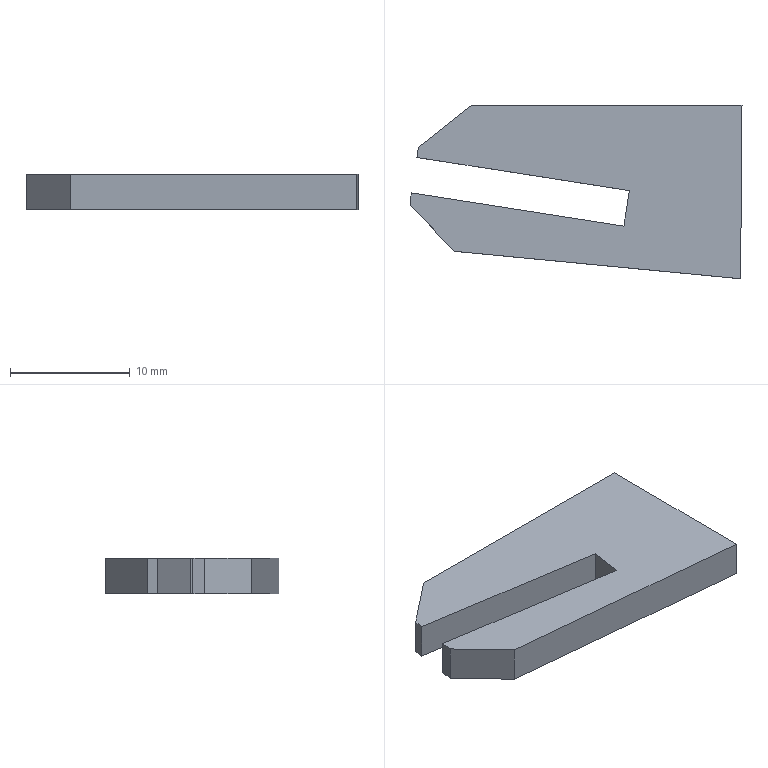Part | SolidWorks | features BaseBody 1 | 1 solid | 12 faces | box 27.749 x 14.503 x 3 mm | volume 877.652 mm3 | plane 12
STEP:
#1=CARTESIAN_POINT('',(-15.417,90.586,-1.5));
#2=VERTEX_POINT('',#1);
#3=CARTESIAN_POINT('',(-19.116,94.481,-1.5));
#4=VERTEX_POINT('',#3);
#5=CARTESIAN_POINT('',(37.126,35.256,-1.5));
#6=DIRECTION('',(-0.6886,0.7251,0.));
#7=VECTOR('',#6,1000.);
#8=LINE('',#5,#7);
#9=EDGE_CURVE('',#2,#4,#8,.T.);
#10=ORIENTED_EDGE('',*,*,#9,.T.);
#11=CARTESIAN_POINT('',(-19.007,95.47,-1.5));
#12=VERTEX_POINT('',#11);
#13=CARTESIAN_POINT('',(-29.164,3.211,-1.5));
#14=DIRECTION('',(0.1094,0.994,0.));
#15=VECTOR('',#14,1000.);
#16=LINE('',#13,#15);
#17=EDGE_CURVE('',#4,#12,#16,.T.);
#18=ORIENTED_EDGE('',*,*,#17,.T.);
#19=CARTESIAN_POINT('',(-1.242,92.691,-1.5));
#20=VERTEX_POINT('',#19);
#21=CARTESIAN_POINT('',(14.126,90.286,-1.5));
#22=DIRECTION('',(0.988,-0.1546,0.));
#23=VECTOR('',#22,1000.);
#24=LINE('',#21,#23);
#25=EDGE_CURVE('',#12,#20,#24,.T.);
#26=ORIENTED_EDGE('',*,*,#25,.T.);
#27=CARTESIAN_POINT('',(-0.7787,95.655,-1.5));
#28=VERTEX_POINT('',#27);
#29=CARTESIAN_POINT('',(-15.369,2.405,-1.5));
#30=DIRECTION('',(-0.1546,-0.988,0.));
#31=VECTOR('',#30,1000.);
#32=LINE('',#29,#31);
#33=EDGE_CURVE('',#28,#20,#32,.T.);
#34=ORIENTED_EDGE('',*,*,#33,.F.);
#35=CARTESIAN_POINT('',(-18.541,98.434,-1.5));
#36=VERTEX_POINT('',#35);
#37=CARTESIAN_POINT('',(14.59,93.25,-1.5));
#38=DIRECTION('',(0.988,-0.1546,0.));
#39=VECTOR('',#38,1000.);
#40=LINE('',#37,#39);
#41=EDGE_CURVE('',#36,#28,#40,.T.);
#42=ORIENTED_EDGE('',*,*,#41,.F.);
#43=CARTESIAN_POINT('',(-18.41,99.272,-1.5));
#44=VERTEX_POINT('',#43);
#45=CARTESIAN_POINT('',(-33.113,5.174,-1.5));
#46=DIRECTION('',(-0.1544,-0.988,0.));
#47=VECTOR('',#46,1000.);
#48=LINE('',#45,#47);
#49=EDGE_CURVE('',#44,#36,#48,.T.);
#50=ORIENTED_EDGE('',*,*,#49,.F.);
#51=CARTESIAN_POINT('',(-13.951,102.794,-1.5));
#52=VERTEX_POINT('',#51);
#53=CARTESIAN_POINT('',(-55.356,70.096,-1.5));
#54=DIRECTION('',(-0.7848,-0.6198,0.));
#55=VECTOR('',#54,1000.);
#56=LINE('',#53,#55);
#57=EDGE_CURVE('',#52,#44,#56,.T.);
#58=ORIENTED_EDGE('',*,*,#57,.F.);
#59=CARTESIAN_POINT('',(8.633,102.795,-1.5));
#60=VERTEX_POINT('',#59);
#61=CARTESIAN_POINT('',(-0.006828,102.795,-1.5));
#62=DIRECTION('',(1.,0.00006642,0.));
#63=VECTOR('',#62,1000.);
#64=LINE('',#61,#63);
#65=EDGE_CURVE('',#52,#60,#64,.T.);
#66=ORIENTED_EDGE('',*,*,#65,.T.);
#67=CARTESIAN_POINT('',(8.515,88.292,-1.5));
#68=VERTEX_POINT('',#67);
#69=CARTESIAN_POINT('',(7.797,-0.06338,-1.5));
#70=DIRECTION('',(0.008129,1.,0.));
#71=VECTOR('',#70,1000.);
#72=LINE('',#69,#71);
#73=EDGE_CURVE('',#68,#60,#72,.T.);
#74=ORIENTED_EDGE('',*,*,#73,.F.);
#75=CARTESIAN_POINT('',(8.464,88.297,-1.5));
#76=DIRECTION('',(0.9954,-0.09542,0.));
#77=VECTOR('',#76,1000.);
#78=LINE('',#75,#77);
#79=EDGE_CURVE('',#2,#68,#78,.T.);
#80=ORIENTED_EDGE('',*,*,#79,.F.);
#81=EDGE_LOOP('',(#10,#18,#26,#34,#42,#50,#58,#66,#74,#80));
#82=FACE_OUTER_BOUND('',#81,.T.);
#83=CARTESIAN_POINT('',(0.,0.,-1.5));
#84=DIRECTION('',(0.,0.,1.));
#85=DIRECTION('',(1.,0.,0.));
#86=AXIS2_PLACEMENT_3D('',#83,#84,#85);
#87=PLANE('',#86);
#88=ADVANCED_FACE('',(#82),#87,.F.);
#89=CARTESIAN_POINT('',(-15.417,90.586,1.5));
#90=VERTEX_POINT('',#89);
#91=CARTESIAN_POINT('',(-19.116,94.481,1.5));
#92=VERTEX_POINT('',#91);
#93=CARTESIAN_POINT('',(37.126,35.256,1.5));
#94=DIRECTION('',(-0.6886,0.7251,0.));
#95=VECTOR('',#94,1000.);
#96=LINE('',#93,#95);
#97=EDGE_CURVE('',#90,#92,#96,.T.);
#98=ORIENTED_EDGE('',*,*,#97,.F.);
#99=CARTESIAN_POINT('',(8.515,88.292,1.5));
#100=VERTEX_POINT('',#99);
#101=CARTESIAN_POINT('',(8.464,88.297,1.5));
#102=DIRECTION('',(0.9954,-0.09542,0.));
#103=VECTOR('',#102,1000.);
#104=LINE('',#101,#103);
#105=EDGE_CURVE('',#90,#100,#104,.T.);
#106=ORIENTED_EDGE('',*,*,#105,.T.);
#107=CARTESIAN_POINT('',(8.633,102.795,1.5));
#108=VERTEX_POINT('',#107);
#109=CARTESIAN_POINT('',(7.797,-0.06338,1.5));
#110=DIRECTION('',(0.008129,1.,0.));
#111=VECTOR('',#110,1000.);
#112=LINE('',#109,#111);
#113=EDGE_CURVE('',#100,#108,#112,.T.);
#114=ORIENTED_EDGE('',*,*,#113,.T.);
#115=CARTESIAN_POINT('',(-13.951,102.794,1.5));
#116=VERTEX_POINT('',#115);
#117=CARTESIAN_POINT('',(-0.006828,102.795,1.5));
#118=DIRECTION('',(1.,0.00006642,0.));
#119=VECTOR('',#118,1000.);
#120=LINE('',#117,#119);
#121=EDGE_CURVE('',#116,#108,#120,.T.);
#122=ORIENTED_EDGE('',*,*,#121,.F.);
#123=CARTESIAN_POINT('',(-18.41,99.272,1.5));
#124=VERTEX_POINT('',#123);
#125=CARTESIAN_POINT('',(-55.356,70.096,1.5));
#126=DIRECTION('',(-0.7848,-0.6198,0.));
#127=VECTOR('',#126,1000.);
#128=LINE('',#125,#127);
#129=EDGE_CURVE('',#116,#124,#128,.T.);
#130=ORIENTED_EDGE('',*,*,#129,.T.);
#131=CARTESIAN_POINT('',(-18.541,98.434,1.5));
#132=VERTEX_POINT('',#131);
#133=CARTESIAN_POINT('',(-33.113,5.174,1.5));
#134=DIRECTION('',(-0.1544,-0.988,0.));
#135=VECTOR('',#134,1000.);
#136=LINE('',#133,#135);
#137=EDGE_CURVE('',#124,#132,#136,.T.);
#138=ORIENTED_EDGE('',*,*,#137,.T.);
#139=CARTESIAN_POINT('',(-0.7787,95.655,1.5));
#140=VERTEX_POINT('',#139);
#141=CARTESIAN_POINT('',(14.59,93.25,1.5));
#142=DIRECTION('',(0.988,-0.1546,0.));
#143=VECTOR('',#142,1000.);
#144=LINE('',#141,#143);
#145=EDGE_CURVE('',#132,#140,#144,.T.);
#146=ORIENTED_EDGE('',*,*,#145,.T.);
#147=CARTESIAN_POINT('',(-1.242,92.691,1.5));
#148=VERTEX_POINT('',#147);
#149=CARTESIAN_POINT('',(-15.369,2.405,1.5));
#150=DIRECTION('',(-0.1546,-0.988,0.));
#151=VECTOR('',#150,1000.);
#152=LINE('',#149,#151);
#153=EDGE_CURVE('',#140,#148,#152,.T.);
#154=ORIENTED_EDGE('',*,*,#153,.T.);
#155=CARTESIAN_POINT('',(-19.007,95.47,1.5));
#156=VERTEX_POINT('',#155);
#157=CARTESIAN_POINT('',(14.126,90.286,1.5));
#158=DIRECTION('',(0.988,-0.1546,0.));
#159=VECTOR('',#158,1000.);
#160=LINE('',#157,#159);
#161=EDGE_CURVE('',#156,#148,#160,.T.);
#162=ORIENTED_EDGE('',*,*,#161,.F.);
#163=CARTESIAN_POINT('',(-29.164,3.211,1.5));
#164=DIRECTION('',(0.1094,0.994,0.));
#165=VECTOR('',#164,1000.);
#166=LINE('',#163,#165);
#167=EDGE_CURVE('',#92,#156,#166,.T.);
#168=ORIENTED_EDGE('',*,*,#167,.F.);
#169=EDGE_LOOP('',(#98,#106,#114,#122,#130,#138,#146,#154,#162,#168));
#170=FACE_OUTER_BOUND('',#169,.T.);
#171=CARTESIAN_POINT('',(0.,0.,1.5));
#172=DIRECTION('',(0.,0.,1.));
#173=DIRECTION('',(1.,0.,0.));
#174=AXIS2_PLACEMENT_3D('',#171,#172,#173);
#175=PLANE('',#174);
#176=ADVANCED_FACE('',(#170),#175,.T.);
#177=ORIENTED_EDGE('',*,*,#17,.F.);
#178=CARTESIAN_POINT('',(-19.116,94.481,1.5));
#179=DIRECTION('',(0.,0.,-1.));
#180=VECTOR('',#179,1000.);
#181=LINE('',#178,#180);
#182=EDGE_CURVE('',#92,#4,#181,.T.);
#183=ORIENTED_EDGE('',*,*,#182,.F.);
#184=ORIENTED_EDGE('',*,*,#167,.T.);
#185=CARTESIAN_POINT('',(-19.007,95.47,1.5));
#186=DIRECTION('',(0.,0.,-1.));
#187=VECTOR('',#186,1000.);
#188=LINE('',#185,#187);
#189=EDGE_CURVE('',#156,#12,#188,.T.);
#190=ORIENTED_EDGE('',*,*,#189,.T.);
#191=EDGE_LOOP('',(#177,#183,#184,#190));
#192=FACE_OUTER_BOUND('',#191,.T.);
#193=CARTESIAN_POINT('',(-29.164,3.211,1.5));
#194=DIRECTION('',(-0.994,0.1094,0.));
#195=DIRECTION('',(0.,0.,1.));
#196=AXIS2_PLACEMENT_3D('',#193,#194,#195);
#197=PLANE('',#196);
#198=ADVANCED_FACE('',(#192),#197,.T.);
#199=ORIENTED_EDGE('',*,*,#25,.F.);
#200=ORIENTED_EDGE('',*,*,#189,.F.);
#201=ORIENTED_EDGE('',*,*,#161,.T.);
#202=CARTESIAN_POINT('',(-1.242,92.691,1.5));
#203=DIRECTION('',(0.,0.,-1.));
#204=VECTOR('',#203,1000.);
#205=LINE('',#202,#204);
#206=EDGE_CURVE('',#148,#20,#205,.T.);
#207=ORIENTED_EDGE('',*,*,#206,.T.);
#208=EDGE_LOOP('',(#199,#200,#201,#207));
#209=FACE_OUTER_BOUND('',#208,.T.);
#210=CARTESIAN_POINT('',(14.126,90.286,1.5));
#211=DIRECTION('',(0.1546,0.988,0.));
#212=DIRECTION('',(0.,0.,-1.));
#213=AXIS2_PLACEMENT_3D('',#210,#211,#212);
#214=PLANE('',#213);
#215=ADVANCED_FACE('',(#209),#214,.T.);
#216=ORIENTED_EDGE('',*,*,#33,.T.);
#217=ORIENTED_EDGE('',*,*,#206,.F.);
#218=ORIENTED_EDGE('',*,*,#153,.F.);
#219=CARTESIAN_POINT('',(-0.7787,95.655,1.5));
#220=DIRECTION('',(0.,0.,-1.));
#221=VECTOR('',#220,1000.);
#222=LINE('',#219,#221);
#223=EDGE_CURVE('',#140,#28,#222,.T.);
#224=ORIENTED_EDGE('',*,*,#223,.T.);
#225=EDGE_LOOP('',(#216,#217,#218,#224));
#226=FACE_OUTER_BOUND('',#225,.T.);
#227=CARTESIAN_POINT('',(-15.369,2.405,1.5));
#228=DIRECTION('',(0.988,-0.1546,0.));
#229=DIRECTION('',(0.,0.,-1.));
#230=AXIS2_PLACEMENT_3D('',#227,#228,#229);
#231=PLANE('',#230);
#232=ADVANCED_FACE('',(#226),#231,.F.);
#233=ORIENTED_EDGE('',*,*,#41,.T.);
#234=ORIENTED_EDGE('',*,*,#223,.F.);
#235=ORIENTED_EDGE('',*,*,#145,.F.);
#236=CARTESIAN_POINT('',(-18.541,98.434,1.5));
#237=DIRECTION('',(0.,0.,-1.));
#238=VECTOR('',#237,1000.);
#239=LINE('',#236,#238);
#240=EDGE_CURVE('',#132,#36,#239,.T.);
#241=ORIENTED_EDGE('',*,*,#240,.T.);
#242=EDGE_LOOP('',(#233,#234,#235,#241));
#243=FACE_OUTER_BOUND('',#242,.T.);
#244=CARTESIAN_POINT('',(14.59,93.25,1.5));
#245=DIRECTION('',(0.1546,0.988,0.));
#246=DIRECTION('',(0.,0.,-1.));
#247=AXIS2_PLACEMENT_3D('',#244,#245,#246);
#248=PLANE('',#247);
#249=ADVANCED_FACE('',(#243),#248,.F.);
#250=ORIENTED_EDGE('',*,*,#49,.T.);
#251=ORIENTED_EDGE('',*,*,#240,.F.);
#252=ORIENTED_EDGE('',*,*,#137,.F.);
#253=CARTESIAN_POINT('',(-18.41,99.272,1.5));
#254=DIRECTION('',(0.,0.,-1.));
#255=VECTOR('',#254,1000.);
#256=LINE('',#253,#255);
#257=EDGE_CURVE('',#124,#44,#256,.T.);
#258=ORIENTED_EDGE('',*,*,#257,.T.);
#259=EDGE_LOOP('',(#250,#251,#252,#258));
#260=FACE_OUTER_BOUND('',#259,.T.);
#261=CARTESIAN_POINT('',(-33.113,5.174,1.5));
#262=DIRECTION('',(0.988,-0.1544,0.));
#263=DIRECTION('',(0.,0.,-1.));
#264=AXIS2_PLACEMENT_3D('',#261,#262,#263);
#265=PLANE('',#264);
#266=ADVANCED_FACE('',(#260),#265,.F.);
#267=ORIENTED_EDGE('',*,*,#57,.T.);
#268=ORIENTED_EDGE('',*,*,#257,.F.);
#269=ORIENTED_EDGE('',*,*,#129,.F.);
#270=CARTESIAN_POINT('',(-13.951,102.794,1.5));
#271=DIRECTION('',(0.,0.,-1.));
#272=VECTOR('',#271,1000.);
#273=LINE('',#270,#272);
#274=EDGE_CURVE('',#116,#52,#273,.T.);
#275=ORIENTED_EDGE('',*,*,#274,.T.);
#276=EDGE_LOOP('',(#267,#268,#269,#275));
#277=FACE_OUTER_BOUND('',#276,.T.);
#278=CARTESIAN_POINT('',(-55.356,70.096,1.5));
#279=DIRECTION('',(0.6198,-0.7848,0.));
#280=DIRECTION('',(0.,0.,-1.));
#281=AXIS2_PLACEMENT_3D('',#278,#279,#280);
#282=PLANE('',#281);
#283=ADVANCED_FACE('',(#277),#282,.F.);
#284=ORIENTED_EDGE('',*,*,#65,.F.);
#285=ORIENTED_EDGE('',*,*,#274,.F.);
#286=ORIENTED_EDGE('',*,*,#121,.T.);
#287=CARTESIAN_POINT('',(8.633,102.795,1.5));
#288=DIRECTION('',(0.,0.,-1.));
#289=VECTOR('',#288,1000.);
#290=LINE('',#287,#289);
#291=EDGE_CURVE('',#108,#60,#290,.T.);
#292=ORIENTED_EDGE('',*,*,#291,.T.);
#293=EDGE_LOOP('',(#284,#285,#286,#292));
#294=FACE_OUTER_BOUND('',#293,.T.);
#295=CARTESIAN_POINT('',(-0.006828,102.795,1.5));
#296=DIRECTION('',(-0.00006642,1.,0.));
#297=DIRECTION('',(0.,0.,1.));
#298=AXIS2_PLACEMENT_3D('',#295,#296,#297);
#299=PLANE('',#298);
#300=ADVANCED_FACE('',(#294),#299,.T.);
#301=ORIENTED_EDGE('',*,*,#73,.T.);
#302=ORIENTED_EDGE('',*,*,#291,.F.);
#303=ORIENTED_EDGE('',*,*,#113,.F.);
#304=CARTESIAN_POINT('',(8.515,88.292,1.5));
#305=DIRECTION('',(0.,0.,-1.));
#306=VECTOR('',#305,1000.);
#307=LINE('',#304,#306);
#308=EDGE_CURVE('',#100,#68,#307,.T.);
#309=ORIENTED_EDGE('',*,*,#308,.T.);
#310=EDGE_LOOP('',(#301,#302,#303,#309));
#311=FACE_OUTER_BOUND('',#310,.T.);
#312=CARTESIAN_POINT('',(7.797,-0.06338,1.5));
#313=DIRECTION('',(-1.,0.008129,0.));
#314=DIRECTION('',(0.,0.,1.));
#315=AXIS2_PLACEMENT_3D('',#312,#313,#314);
#316=PLANE('',#315);
#317=ADVANCED_FACE('',(#311),#316,.F.);
#318=ORIENTED_EDGE('',*,*,#79,.T.);
#319=ORIENTED_EDGE('',*,*,#308,.F.);
#320=ORIENTED_EDGE('',*,*,#105,.F.);
#321=CARTESIAN_POINT('',(-15.417,90.586,1.5));
#322=DIRECTION('',(0.,0.,-1.));
#323=VECTOR('',#322,1000.);
#324=LINE('',#321,#323);
#325=EDGE_CURVE('',#90,#2,#324,.T.);
#326=ORIENTED_EDGE('',*,*,#325,.T.);
#327=EDGE_LOOP('',(#318,#319,#320,#326));
#328=FACE_OUTER_BOUND('',#327,.T.);
#329=CARTESIAN_POINT('',(8.464,88.297,1.5));
#330=DIRECTION('',(0.09542,0.9954,0.));
#331=DIRECTION('',(0.,0.,-1.));
#332=AXIS2_PLACEMENT_3D('',#329,#330,#331);
#333=PLANE('',#332);
#334=ADVANCED_FACE('',(#328),#333,.F.);
#335=ORIENTED_EDGE('',*,*,#9,.F.);
#336=ORIENTED_EDGE('',*,*,#325,.F.);
#337=ORIENTED_EDGE('',*,*,#97,.T.);
#338=ORIENTED_EDGE('',*,*,#182,.T.);
#339=EDGE_LOOP('',(#335,#336,#337,#338));
#340=FACE_OUTER_BOUND('',#339,.T.);
#341=CARTESIAN_POINT('',(37.126,35.256,1.5));
#342=DIRECTION('',(-0.7251,-0.6886,0.));
#343=DIRECTION('',(-0.6886,0.7251,0.));
#344=AXIS2_PLACEMENT_3D('',#341,#342,#343);
#345=PLANE('',#344);
#346=ADVANCED_FACE('',(#340),#345,.T.);
#347=CLOSED_SHELL('',(#88,#176,#198,#215,#232,#249,#266,#283,#300,#317,#334,#346));
#348=MANIFOLD_SOLID_BREP('',#347);
#349=CARTESIAN_POINT('',(0.,0.,0.));
#350=DIRECTION('',(0.,0.,1.));
#351=DIRECTION('',(1.,0.,0.));
#352=AXIS2_PLACEMENT_3D('',#349,#350,#351);
#353=(LENGTH_UNIT()NAMED_UNIT(*)SI_UNIT(.MILLI.,.METRE.));
#354=UNCERTAINTY_MEASURE_WITH_UNIT(LENGTH_MEASURE(0.00001),#353,'','');
#355=(NAMED_UNIT(*)PLANE_ANGLE_UNIT()SI_UNIT($,.RADIAN.));
#356=(NAMED_UNIT(*)SI_UNIT($,.STERADIAN.)SOLID_ANGLE_UNIT());
#357=(GEOMETRIC_REPRESENTATION_CONTEXT(3)GLOBAL_UNCERTAINTY_ASSIGNED_CONTEXT((#354))GLOBAL_UNIT_ASSIGNED_CONTEXT((#353,#355,#356))REPRESENTATION_CONTEXT('',''));
#358=ADVANCED_BREP_SHAPE_REPRESENTATION('',(#348,#352),#357);